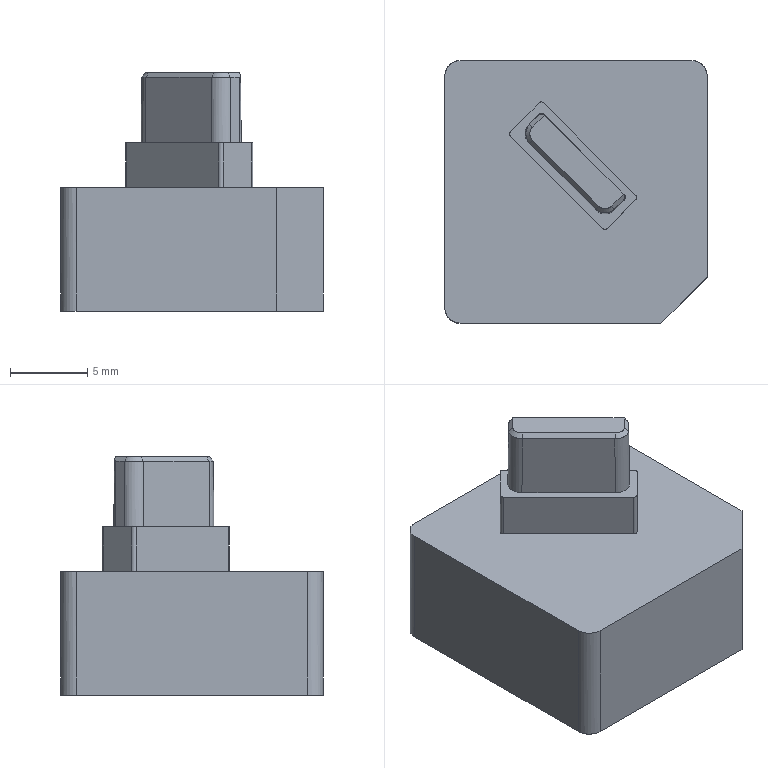NC program | PowerMill | posted with a generic post | part box 17 x 17 x 15.424 mm
Lines 1 to 1056 of 38437:
%
O0001
N104 ( POWERMILL CB  : 2026004.0)
N105 ( POST VER      : 2026.0.0.5161)
N106 ( OPTION FILE   : FANUC)
N107 ( OUTPUT WORKPLANE : WORLD)
N108 (  )
N109 ( TOOL LIST )
N110 (---------------------------------------)
N111 ( NO. | ID        | DIA.| TIP RAD|LENGTH)
N112 (---------------------------------------)
N113 (    1|D10C_1_1   |10.0 |  0.0   |70.88 )
N114 (    3|D10_1_1    |10.0 |  0.0   | 70.6 )
N115 (   14|D4_1_1     | 4.0 |  0.0   | 62.6 )
N116 (   13|TEXT_D4_1_1| 4.0 |  0.3   |62.68 )
N117 (---------------------------------------)
N118 (  )
N119 ( NUMBER OF TOOLPATHS: 10.0 )
N120 ( ESTIMATED PROGRAM DURATION: 0 HOURS 4 MIN 27 SEC)
N121 (  )
N122 G00 G21 G80 G40 G17
N123 G90
N124 G54
N125 G53 Z0.0
N126 (---------------)
N127 ( START TOOLPATH : 精公开粗01-扫面平行-D10C )
N128 (---------------)
N129 ( TOOL NO.    :1 )
N130 ( TOOL TYPE   : ENDMILL)
N131 ( TOOL ID     : D10C_1_1)
N132 ( TOOL DIA    : 10.0 LENGTH 70.88)
N133 T1
N134 M6
N135 S8000 M03
N136 G00 G90 X0.0 Y0.0
N137 G43 Z10.2 H1
N138
N139 G05 P10000 R4
N140 X11.28 Y11.28
N141 Z1.134
N142 G01 Z-0.066 F6000.0
N143 X-11.28 F10000.0
N144 Y5.64
N145 X11.28
N146 Y0.0
N147 X-11.28
N148 Y-5.64
N149 X11.28
N150 Y-11.28
N151 X-11.28
N152 X-16.28
N153 G00 Z10.2
N154 G05 P0
N155 (---------------)
N156 ( END TOOLPATH : 精公开粗01-扫面平行-D10C )
N157 (---------------)
N158 ( START TOOLPATH : 精公开粗01-外形偏置-D10C )
N159 (---------------)
N160 G00 X-0.181 Y1.1575 Z9.884
N161 G05 P10000 R4
N162 X16.993 Y4.7643
N163 Z0.7104
N164 G01 Z-0.4896 F6000.0
N165 X16.4655 F10000.0
N166 G03 X11.718 Y0.0168 I0.0 J-4.7475
N167 G01 Y-10.28
N168 G02 X10.718 Y-11.28 I-1.0 J0.0
N169 G01 X-11.08
N170 G02 X-12.08 Y-10.28 I0.0 J1.0
N171 G01 Y12.595
N172 G02 X-11.08 Y13.595 I1.0 J0.0
N173 G01 X10.718
N174 G02 X11.718 Y12.595 I0.0 J-1.0
N175 G01 Y0.0168
N176 X8.404 Y-0.196
N177 X8.4164 Y-0.3894
N178 X8.3267 Y-1.3785
N179 X8.1894 Y-1.9362
N180 X7.8985 Y-2.7096
N181 X7.5533 Y-3.3402
N182 X6.8288 Y-4.2565
N183 X6.0064 Y-5.075
N184 X5.233 Y-5.6668
N185 X5.0107 Y-5.8033
N186 X4.4596 Y-6.0808
N187 X3.6861 Y-6.3853
N188 X2.8628 Y-6.5768
N189 X2.1393 Y-6.649
N190 X1.3659 Y-6.6271
N191 X0.5924 Y-6.5194
N192 X-0.181 Y-6.3016
N193 X-0.9544 Y-5.9651
N194 X-1.2535 Y-5.8033
N195 X-1.7279 Y-5.4941
N196 X-2.2951 Y-5.0299
N197 X-2.5013 Y-4.8324
N198 X-6.171 Y-1.1628
N199 X-7.1418 Y-0.1514
N200 X-7.5329 Y0.3841
N201 X-7.9153 Y1.0674
N202 X-8.2576 Y1.9309
N203 X-8.4393 Y2.7044
N204 X-8.5261 Y3.4778
N205 X-8.5038 Y4.2512
N206 X-8.4011 Y5.0246
N207 X-8.1855 Y5.7981
N208 X-7.9153 Y6.4478
N209 X-7.3844 Y7.3449
N210 X-7.1418 Y7.664
N211 X-6.7331 Y8.1183
N212 X-5.9378 Y8.8918
N213 X-5.595 Y9.1738
N214 X-4.8222 Y9.6652
N215 X-4.0481 Y9.9937
N216 X-3.2747 Y10.1962
N217 X-2.5013 Y10.2908
N218 X-1.7279 Y10.2681
N219 X-0.9544 Y10.1475
N220 X-0.181 Y9.9029
N221 X0.3303 Y9.6652
N222 X0.5924 Y9.5152
N223 X1.3659 Y8.9732
N224 X2.1393 Y8.2277
N225 X6.8887 Y3.4778
N226 X7.4928 Y2.7044
N227 X7.9241 Y1.9309
N228 X8.2071 Y1.1575
N229 X8.3668 Y0.3841
N230 X8.404 Y-0.196
N231 X11.718 Y0.0168
N232 G00 Z3.3368
N233 G01 X16.993 Y4.7643
N234 G00 Z0.3368
N235 G01 Z-0.8632 F6000.0
N236 X16.4655 F10000.0
N237 G03 X11.718 Y0.0168 I0.0 J-4.7475
N238 G01 Y-10.28
N239 G02 X10.718 Y-11.28 I-1.0 J0.0
N240 G01 X-11.08
N241 G02 X-12.08 Y-10.28 I0.0 J1.0
N242 G01 Y12.595
N243 G02 X-11.08 Y13.595 I1.0 J0.0
N244 G01 X10.718
N245 G02 X11.718 Y12.595 I0.0 J-1.0
N246 G01 Y0.0239
N247 X8.4111 Y-0.196
N248 X8.424 Y-0.3894
N249 X8.3643 Y-1.1628
N250 X8.3328 Y-1.3101
N251 X8.3266 Y-1.3785
N252 X8.2632 Y-1.6361
N253 X8.1991 Y-1.9362
N254 X7.9038 Y-2.7096
N255 X7.5533 Y-3.3517
N256 X6.8433 Y-4.2565
N257 X6.0626 Y-5.0299
N258 X6.015 Y-5.0664
N259 X6.0064 Y-5.075
N260 X5.2793 Y-5.6313
N261 X5.233 Y-5.6668
N262 X5.231 Y-5.6679
N263 X5.0106 Y-5.8033
N264 X4.7463 Y-5.9364
N265 X4.4596 Y-6.0952
N266 X3.6861 Y-6.3853
N267 X2.8923 Y-6.5768
N268 X2.1393 Y-6.6513
N269 X1.3659 Y-6.6355
N270 X0.5924 Y-6.5238
N271 X-0.181 Y-6.3016
N272 X-0.9544 Y-5.9721
N273 X-1.2585 Y-5.8033
N274 X-1.7279 Y-5.4944
N275 X-2.3045 Y-5.0299
N276 X-2.5013 Y-4.8411
N277 X-6.3684 Y-0.9749
N278 X-6.9415 Y-0.3894
N279 X-7.1418 Y-0.1528
N280 X-7.5329 Y0.3841
N281 X-7.9153 Y1.052
N282 X-8.2576 Y1.9309
N283 X-8.4465 Y2.7044
N284 X-8.5286 Y3.4778
N285 X-8.5153 Y4.2512
N286 X-8.4055 Y5.0246
N287 X-8.1856 Y5.7981
N288 X-7.9153 Y6.4608
N289 X-7.3847 Y7.3449
N290 X-7.1418 Y7.6656
N291 X-6.7378 Y8.1183
N292 X-5.9501 Y8.8918
N293 X-5.595 Y9.1789
N294 X-4.8282 Y9.6652
N295 X-4.0481 Y10.0018
N296 X-3.2747 Y10.2057
N297 X-2.5013 Y10.2955
N298 X-1.7279 Y10.2743
N299 X-0.9544 Y10.1526
N300 X-0.181 Y9.9068
N301 X-0.0726 Y9.8524
N302 X0.3303 Y9.6651
N303 X0.5395 Y9.5454
N304 X0.5924 Y9.5189
N305 X1.3659 Y8.9797
N306 X2.1393 Y8.2347
N307 X6.8933 Y3.4778
N308 X7.499 Y2.7044
N309 X7.9275 Y1.9309
N310 X8.2137 Y1.1575
N311 X8.3726 Y0.3841
N312 X8.4111 Y-0.196
N313 X11.718 Y0.0239
N314 Y0.0168
N315 G00 Z2.9632
N316 G01 X16.993 Y4.7643
N317 G00 Z-0.0368
N318 G01 Z-1.2368 F6000.0
N319 X16.4655 F10000.0
N320 G03 X11.718 Y0.0168 I0.0 J-4.7475
N321 G01 Y-10.28
N322 G02 X10.718 Y-11.28 I-1.0 J0.0
N323 G01 X-11.08
N324 G02 X-12.08 Y-10.28 I0.0 J1.0
N325 G01 Y12.595
N326 G02 X-11.08 Y13.595 I1.0 J0.0
N327 G01 X10.718
N328 G02 X11.718 Y12.595 I0.0 J-1.0
N329 G01 Y0.0198
N330 X8.4151 Y-0.196
N331 X8.4277 Y-0.3894
N332 X8.3702 Y-1.1628
N333 X8.3286 Y-1.3561
N334 X8.3266 Y-1.3785
N335 X8.3044 Y-1.4688
N336 X8.2037 Y-1.9362
N337 X7.9091 Y-2.7096
N338 X7.5533 Y-3.3585
N339 X6.8479 Y-4.2565
N340 X6.0675 Y-5.0299
N341 X5.233 Y-5.6696
N342 X5.1815 Y-5.6983
N343 X5.0106 Y-5.8033
N344 X4.8222 Y-5.8981
N345 X4.4596 Y-6.0998
N346 X3.6861 Y-6.3854
N347 X2.9192 Y-6.5768
N348 X2.1393 Y-6.6536
N349 X1.3659 Y-6.6409
N350 X0.5924 Y-6.5284
N351 X-0.181 Y-6.3024
N352 X-0.9544 Y-5.978
N353 X-1.2661 Y-5.8033
N354 X-1.7279 Y-5.4946
N355 X-2.3103 Y-5.0299
N356 X-2.5013 Y-4.8467
N357 X-6.1852 Y-1.1628
N358 X-6.9467 Y-0.3894
N359 X-7.1418 Y-0.1583
N360 X-7.5353 Y0.3841
N361 X-7.9153 Y1.0427
N362 X-8.2577 Y1.9309
N363 X-8.4526 Y2.7044
N364 X-8.531 Y3.4778
N365 X-8.5199 Y4.2512
N366 X-8.4101 Y5.0246
N367 X-8.186 Y5.7981
N368 X-7.9153 Y6.4701
N369 X-7.385 Y7.3449
N370 X-7.1418 Y7.6711
N371 X-6.7424 Y8.1183
N372 X-5.9553 Y8.8918
N373 X-5.595 Y9.1838
N374 X-4.8345 Y9.6652
N375 X-4.0481 Y10.0064
N376 X-3.2747 Y10.2103
N377 X-2.5013 Y10.3002
N378 X-1.7279 Y10.2796
N379 X-0.9544 Y10.1573
N380 X-0.181 Y9.9114
N381 X0.0543 Y9.7934
N382 X0.3303 Y9.6651
N383 X0.4735 Y9.5831
N384 X0.5924 Y9.5235
N385 X1.3659 Y8.9843
N386 X2.1393 Y8.2393
N387 X6.8979 Y3.4778
N388 X7.5036 Y2.7044
N389 X7.9321 Y1.9309
N390 X8.2188 Y1.1575
N391 X8.3772 Y0.3841
N392 X8.4151 Y-0.196
N393 X11.718 Y0.0198
N394 Y0.0168
N395 G00 Z2.5896
N396 G01 X16.993 Y4.7643
N397 G00 Z-0.4104
N398 G01 Z-1.6104 F6000.0
N399 X16.4655 F10000.0
N400 G03 X11.718 Y0.0168 I0.0 J-4.7475
N401 G01 Y0.0156
N402 X8.419 Y-0.196
N403 X8.4314 Y-0.3894
N404 X8.3748 Y-1.1628
N405 X8.2083 Y-1.9362
N406 X7.9123 Y-2.7096
N407 X7.5533 Y-3.3651
N408 X6.8526 Y-4.2565
N409 X6.0725 Y-5.0299
N410 X5.233 Y-5.6742
N411 X5.1012 Y-5.7475
N412 X5.0106 Y-5.8032
N413 X4.9106 Y-5.8535
N414 X4.4596 Y-6.1044
N415 X3.6861 Y-6.3889
N416 X2.9447 Y-6.5768
N417 X2.1393 Y-6.6572
N418 X1.3659 Y-6.6455
N419 X0.5924 Y-6.533
N420 X-0.181 Y-6.307
N421 X-0.9544 Y-5.9826
N422 X-1.2737 Y-5.8033
N423 X-1.7279 Y-5.4967
N424 X-2.3152 Y-5.0299
N425 X-2.5013 Y-4.8513
N426 X-6.1898 Y-1.1628
N427 X-6.9512 Y-0.3894
N428 X-7.1418 Y-0.1637
N429 X-7.5399 Y0.3841
N430 X-7.9153 Y1.0334
N431 X-8.2609 Y1.9309
N432 X-8.4572 Y2.7044
N433 X-8.5346 Y3.4778
N434 X-8.5245 Y4.2512
N435 X-8.4147 Y5.0246
N436 X-8.1906 Y5.7981
N437 X-7.9153 Y6.4795
N438 X-7.3872 Y7.3449
N439 X-7.1418 Y7.6765
N440 X-6.747 Y8.1183
N441 X-5.9605 Y8.8918
N442 X-5.595 Y9.1884
N443 X-4.8408 Y9.6652
N444 X-4.0481 Y10.011
N445 X-3.2747 Y10.2149
N446 X-2.5013 Y10.3044
N447 X-1.7279 Y10.2842
N448 X-0.9544 Y10.162
N449 X-0.181 Y9.916
N450 X0.1813 Y9.7343
N451 X0.3302 Y9.6651
N452 X0.4076 Y9.6208
N453 X0.5924 Y9.5281
N454 X1.3659 Y8.9889
N455 X2.1393 Y8.2439
N456 X6.9025 Y3.4778
N457 X7.5082 Y2.7044
N458 X7.9367 Y1.9309
N459 X8.2234 Y1.1575
N460 X8.3818 Y0.3841
N461 X8.419 Y-0.196
N462 X11.718 Y0.0156
N463 Y-10.28
N464 G02 X10.718 Y-11.28 I-1.0 J0.0
N465 G01 X-11.08
N466 G02 X-12.08 Y-10.28 I0.0 J1.0
N467 G01 Y12.595
N468 G02 X-11.08 Y13.595 I1.0 J0.0
N469 G01 X10.718
N470 G02 X11.718 Y12.595 I0.0 J-1.0
N471 G01 Y0.0168
N472 G00 Z2.216
N473 G01 X16.993 Y4.7643
N474 G00 Z-0.784
N475 G01 Z-1.984 F6000.0
N476 X16.4655 F10000.0
N477 G03 X11.718 Y0.0168 I0.0 J-4.7475
N478 G01 Y0.0114
N479 X8.4229 Y-0.196
N480 X8.4351 Y-0.3894
N481 X8.3795 Y-1.1628
N482 X8.2129 Y-1.9362
N483 X7.9169 Y-2.7096
N484 X7.5533 Y-3.3718
N485 X6.8572 Y-4.2565
N486 X6.0774 Y-5.0299
N487 X5.233 Y-5.6789
N488 X5.0209 Y-5.7968
N489 X5.0106 Y-5.8032
N490 X4.9991 Y-5.8089
N491 X4.4596 Y-6.109
N492 X3.6861 Y-6.3935
N493 X2.9701 Y-6.5768
N494 X2.1393 Y-6.6618
N495 X1.3659 Y-6.6501
N496 X0.7874 Y-6.5768
N497 X0.6667 Y-6.5437
N498 X0.5924 Y-6.5329
N499 X0.073 Y-6.3812
N500 X-0.181 Y-6.3116
N501 X-0.9544 Y-5.9872
N502 X-1.2812 Y-5.8033
N503 X-1.7279 Y-5.5009
N504 X-2.3202 Y-5.0299
N505 X-2.5013 Y-4.8559
N506 X-6.1944 Y-1.1628
N507 X-6.9557 Y-0.3894
N508 X-6.9972 Y-0.3348
N509 X-7.1418 Y-0.1637
N510 X-7.4418 Y0.2491
N511 X-7.5445 Y0.3841
N512 X-7.9153 Y1.024
N513 X-8.2655 Y1.9309
N514 X-8.4618 Y2.7044
N515 X-8.5392 Y3.4778
N516 X-8.5291 Y4.2512
N517 X-8.4193 Y5.0246
N518 X-8.1952 Y5.7981
N519 X-7.9153 Y6.4888
N520 X-7.3914 Y7.3449
N521 X-7.1418 Y7.6819
N522 X-6.7516 Y8.1183
N523 X-5.9657 Y8.8918
N524 X-5.595 Y9.193
N525 X-4.8472 Y9.6652
N526 X-4.0481 Y10.0156
N527 X-3.2747 Y10.2196
N528 X-2.5013 Y10.3083
N529 X-1.7279 Y10.2888
N530 X-0.9544 Y10.1666
N531 X-0.181 Y9.9206
N532 X0.3083 Y9.6752
N533 X0.3302 Y9.665
N534 X0.3416 Y9.6585
N535 X0.5924 Y9.5327
N536 X1.3659 Y8.9935
N537 X2.1393 Y8.2485
N538 X6.9071 Y3.4778
N539 X7.5128 Y2.7044
N540 X7.9413 Y1.9309
N541 X8.228 Y1.1575
N542 X8.3864 Y0.3841
N543 X8.4229 Y-0.196
N544 X11.718 Y0.0114
N545 Y-10.28
N546 G02 X10.718 Y-11.28 I-1.0 J0.0
N547 G01 X-11.08
N548 G02 X-12.08 Y-10.28 I0.0 J1.0
N549 G01 Y12.595
N550 G02 X-11.08 Y13.595 I1.0 J0.0
N551 G01 X10.718
N552 G02 X11.718 Y12.595 I0.0 J-1.0
N553 G01 Y0.0168
N554 G00 Z1.8424
N555 G01 X16.993 Y4.7643
N556 G00 Z-1.1576
N557 G01 Z-2.3576 F6000.0
N558 X16.4655 F10000.0
N559 G03 X11.718 Y0.0168 I0.0 J-4.7475
N560 G01 Y0.0072
N561 X8.4268 Y-0.196
N562 X8.4387 Y-0.3894
N563 X8.3841 Y-1.1628
N564 X8.2175 Y-1.9362
N565 X7.9215 Y-2.7096
N566 X7.5533 Y-3.3784
N567 X6.8618 Y-4.2565
N568 X6.0823 Y-5.0299
N569 X5.233 Y-5.6835
N570 X4.4596 Y-6.1136
N571 X3.6861 Y-6.3982
N572 X2.9956 Y-6.5768
N573 X2.1393 Y-6.6664
N574 X1.3659 Y-6.6547
N575 X0.7622 Y-6.5768
N576 X0.6154 Y-6.5362
N577 X0.5924 Y-6.5329
N578 X0.404 Y-6.4778
N579 X-0.181 Y-6.3162
N580 X-0.9544 Y-5.9918
N581 X-1.2888 Y-5.8033
N582 X-1.7279 Y-5.5051
N583 X-2.3251 Y-5.0299
N584 X-2.5013 Y-4.8605
N585 X-6.199 Y-1.1628
N586 X-6.9602 Y-0.3894
N587 X-7.0434 Y-0.2801
N588 X-7.1418 Y-0.1637
N589 X-7.3446 Y0.1154
N590 X-7.5491 Y0.3841
N591 X-7.9153 Y1.0147
N592 X-8.2701 Y1.9309
N593 X-8.4664 Y2.7044
N594 X-8.5438 Y3.4778
N595 X-8.5337 Y4.2512
N596 X-8.4239 Y5.0246
N597 X-8.1998 Y5.7981
N598 X-7.9153 Y6.4981
N599 X-7.3956 Y7.3449
N600 X-7.1418 Y7.6874
N601 X-6.7562 Y8.1183
N602 X-5.9709 Y8.8918
N603 X-5.595 Y9.1976
N604 X-4.8535 Y9.6652
N605 X-4.0481 Y10.0202
N606 X-3.2747 Y10.2242
N607 X-2.5013 Y10.3123
N608 X-1.7279 Y10.2934
N609 X-0.9544 Y10.1712
N610 X-0.181 Y9.9252
N611 X0.5924 Y9.5373
N612 X1.3659 Y8.9982
N613 X2.1393 Y8.2532
N614 X6.9118 Y3.4778
N615 X7.5174 Y2.7044
N616 X7.946 Y1.9309
N617 X8.2326 Y1.1575
N618 X8.391 Y0.3841
N619 X8.4268 Y-0.196
N620 X11.718 Y0.0072
N621 Y-10.28
N622 G02 X10.718 Y-11.28 I-1.0 J0.0
N623 G01 X-11.08
N624 G02 X-12.08 Y-10.28 I0.0 J1.0
N625 G01 Y12.595
N626 G02 X-11.08 Y13.595 I1.0 J0.0
N627 G01 X10.718
N628 G02 X11.718 Y12.595 I0.0 J-1.0
N629 G01 Y0.0168
N630 G00 Z1.4688
N631 G01 X16.993 Y4.7643
N632 G00 Z-1.5312
N633 G01 Z-2.7312 F6000.0
N634 X16.4655 F10000.0
N635 G03 X11.718 Y0.0168 I0.0 J-4.7475
N636 G01 Y0.0029
N637 X8.4307 Y-0.196
N638 X8.4424 Y-0.3894
N639 X8.3887 Y-1.1628
N640 X8.2222 Y-1.9362
N641 X7.9261 Y-2.7096
N642 X7.5533 Y-3.3851
N643 X6.8664 Y-4.2565
N644 X6.0872 Y-5.0299
N645 X5.233 Y-5.6881
N646 X4.4596 Y-6.1182
N647 X3.6861 Y-6.4028
N648 X3.0199 Y-6.5768
N649 X2.1393 Y-6.671
N650 X1.3659 Y-6.6593
N651 X0.7371 Y-6.5768
N652 X-0.181 Y-6.3208
N653 X-0.9544 Y-5.9964
N654 X-1.2964 Y-5.8033
N655 X-1.7279 Y-5.5094
N656 X-2.33 Y-5.0299
N657 X-2.5013 Y-4.8651
N658 X-6.2036 Y-1.1628
N659 X-6.9647 Y-0.3894
N660 X-7.0897 Y-0.2252
N661 X-7.1417 Y-0.1636
N662 X-7.2482 Y-0.0171
N663 X-7.5538 Y0.3841
N664 X-7.9153 Y1.0053
N665 X-8.2747 Y1.9309
N666 X-8.4711 Y2.7044
N667 X-8.5484 Y3.4778
N668 X-8.5383 Y4.2512
N669 X-8.4285 Y5.0246
N670 X-8.2045 Y5.7981
N671 X-7.9153 Y6.5075
N672 X-7.4002 Y7.3449
N673 X-7.1418 Y7.6928
N674 X-6.7608 Y8.1183
N675 X-5.976 Y8.8918
N676 X-5.595 Y9.2022
N677 X-4.8598 Y9.6652
N678 X-4.0481 Y10.0248
N679 X-3.2747 Y10.2288
N680 X-2.5013 Y10.3163
N681 X-1.7279 Y10.298
N682 X-0.9544 Y10.1758
N683 X-0.181 Y9.9298
N684 X0.5924 Y9.5419
N685 X1.3659 Y9.0028
N686 X2.1393 Y8.2578
N687 X6.9164 Y3.4778
N688 X7.522 Y2.7044
N689 X7.9506 Y1.9309
N690 X8.2373 Y1.1575
N691 X8.3956 Y0.3841
N692 X8.4307 Y-0.196
N693 X11.718 Y0.0029
N694 Y-10.28
N695 G02 X10.718 Y-11.28 I-1.0 J0.0
N696 G01 X-11.08
N697 G02 X-12.08 Y-10.28 I0.0 J1.0
N698 G01 Y12.595
N699 G02 X-11.08 Y13.595 I1.0 J0.0
N700 G01 X10.718
N701 G02 X11.718 Y12.595 I0.0 J-1.0
N702 G01 Y0.0168
N703 G00 Z1.0952
N704 G01 X16.993 Y4.7643
N705 G00 Z-1.9048
N706 G01 Z-3.1048 F6000.0
N707 X16.4655 F10000.0
N708 G03 X11.718 Y0.0168 I0.0 J-4.7475
N709 G01 Y-0.0014
N710 X8.4346 Y-0.196
N711 X8.4461 Y-0.3894
N712 X8.3933 Y-1.1628
N713 X8.2268 Y-1.9362
N714 X7.9307 Y-2.7096
N715 X7.5533 Y-3.3918
N716 X6.871 Y-4.2565
N717 X6.0922 Y-5.0299
N718 X5.233 Y-5.6927
N719 X4.4596 Y-6.1228
N720 X3.6861 Y-6.4074
N721 X3.0429 Y-6.5768
N722 X2.1393 Y-6.6757
N723 X1.3659 Y-6.6639
N724 X0.7141 Y-6.5768
N725 X-0.181 Y-6.3254
N726 X-0.9544 Y-6.001
N727 X-1.3039 Y-5.8033
N728 X-1.7279 Y-5.514
N729 X-2.3349 Y-5.0299
N730 X-2.4672 Y-4.8978
N731 X-2.5012 Y-4.8651
N732 X-3.2744 Y-4.0919
N733 X-6.2082 Y-1.1628
N734 X-6.9692 Y-0.3894
N735 X-7.1362 Y-0.17
N736 X-7.1417 Y-0.1636
N737 X-7.1527 Y-0.1484
N738 X-7.5584 Y0.3841
N739 X-7.9153 Y0.996
N740 X-8.2793 Y1.9309
N741 X-8.4757 Y2.7044
N742 X-8.553 Y3.4778
N743 X-8.5429 Y4.2512
N744 X-8.4331 Y5.0246
N745 X-8.2091 Y5.7981
N746 X-7.9153 Y6.5168
N747 X-7.4048 Y7.3449
N748 X-7.1418 Y7.6982
N749 X-6.7654 Y8.1183
N750 X-5.9812 Y8.8918
N751 X-5.595 Y9.2068
N752 X-4.8669 Y9.6652
N753 X-4.0481 Y10.0295
N754 X-3.2747 Y10.2334
N755 X-2.5013 Y10.3203
N756 X-1.7279 Y10.3026
N757 X-0.9544 Y10.1804
N758 X-0.181 Y9.9344
N759 X0.5924 Y9.5465
N760 X1.3659 Y9.0074
N761 X2.1393 Y8.2624
N762 X6.921 Y3.4778
N763 X7.5267 Y2.7044
N764 X7.9552 Y1.9309
N765 X8.2419 Y1.1575
N766 X8.4002 Y0.3841
N767 X8.4346 Y-0.196
N768 X11.718 Y-0.0014
N769 Y-10.28
N770 G02 X10.718 Y-11.28 I-1.0 J0.0
N771 G01 X-11.08
N772 G02 X-12.08 Y-10.28 I0.0 J1.0
N773 G01 Y12.595
N774 G02 X-11.08 Y13.595 I1.0 J0.0
N775 G01 X10.718
N776 G02 X11.718 Y12.595 I0.0 J-1.0
N777 G01 Y0.0168
N778 G00 Z0.7216
N779 G01 X16.993 Y4.7643
N780 G00 Z-2.2784
N781 G01 Z-3.4784 F6000.0
N782 X16.4655 F10000.0
N783 G03 X11.718 Y0.0168 I0.0 J-4.7475
N784 G01 Y-0.0058
N785 X8.4385 Y-0.196
N786 X8.4497 Y-0.3894
N787 X8.3979 Y-1.1628
N788 X8.2314 Y-1.9362
N789 X7.9353 Y-2.7096
N790 X7.5533 Y-3.3984
N791 X6.8756 Y-4.2565
N792 X6.0971 Y-5.0299
N793 X5.233 Y-5.6973
N794 X4.4596 Y-6.1274
N795 X3.6861 Y-6.412
N796 X3.066 Y-6.5768
N797 X2.1393 Y-6.6803
N798 X1.3659 Y-6.6685
N799 X0.6916 Y-6.5768
N800 X-0.181 Y-6.33
N801 X-0.9544 Y-6.0056
N802 X-1.3114 Y-5.8033
N803 X-1.7279 Y-5.5186
N804 X-2.3398 Y-5.0299
N805 X-6.2129 Y-1.1628
N806 X-6.9737 Y-0.3894
N807 X-7.563 Y0.3841
N808 X-7.9153 Y0.9867
N809 X-8.2839 Y1.9309
N810 X-8.4803 Y2.7044
N811 X-8.5576 Y3.4778
N812 X-8.5476 Y4.2512
N813 X-8.4377 Y5.0246
N814 X-8.2137 Y5.7981
N815 X-7.9153 Y6.5261
N816 X-7.4094 Y7.3449
N817 X-7.1418 Y7.7036
N818 X-6.77 Y8.1183
N819 X-5.9863 Y8.8918
N820 X-5.595 Y9.2114
N821 X-4.8752 Y9.6652
N822 X-4.0481 Y10.0341
N823 X-3.2747 Y10.238
N824 X-2.5013 Y10.3242
N825 X-1.7279 Y10.3072
N826 X-0.9544 Y10.185
N827 X-0.181 Y9.9391
N828 X0.5924 Y9.5511
N829 X1.3659 Y9.012
N830 X2.1393 Y8.267
N831 X6.9256 Y3.4778
N832 X7.5313 Y2.7044
N833 X7.9598 Y1.9309
N834 X8.2465 Y1.1575
N835 X8.4048 Y0.3841
N836 X8.4385 Y-0.196
N837 X11.718 Y-0.0058
N838 Y-10.28
N839 G02 X10.718 Y-11.28 I-1.0 J0.0
N840 G01 X-11.08
N841 G02 X-12.08 Y-10.28 I0.0 J1.0
N842 G01 Y12.595
N843 G02 X-11.08 Y13.595 I1.0 J0.0
N844 G01 X10.718
N845 G02 X11.718 Y12.595 I0.0 J-1.0
N846 G01 Y0.0168
N847 G00 Z0.348
N848 G01 X16.993 Y4.7643
N849 G00 Z-2.652
N850 G01 Z-3.852 F6000.0
N851 X16.4655 F10000.0
N852 G03 X11.718 Y0.0168 I0.0 J-4.7475
N853 G01 Y-0.1071
N854 X8.4478 Y-0.2927
N855 X8.4533 Y-0.3894
N856 X8.4025 Y-1.1628
N857 X8.236 Y-1.9362
N858 X7.94 Y-2.7096
N859 X7.5533 Y-3.4051
N860 X6.8802 Y-4.2565
N861 X6.102 Y-5.0299
N862 X5.233 Y-5.7019
N863 X4.4596 Y-6.1321
N864 X3.6861 Y-6.4166
N865 X3.0891 Y-6.5768
N866 X2.1393 Y-6.6849
N867 X1.3659 Y-6.6732
N868 X0.6691 Y-6.5768
N869 X-0.181 Y-6.3347
N870 X-0.9544 Y-6.0102
N871 X-1.3188 Y-5.8033
N872 X-1.7279 Y-5.5232
N873 X-2.3447 Y-5.0299
N874 X-6.2175 Y-1.1628
N875 X-6.9781 Y-0.3894
N876 X-7.5676 Y0.3841
N877 X-7.9153 Y0.9773
N878 X-8.2885 Y1.9309
N879 X-8.4849 Y2.7044
N880 X-8.5622 Y3.4778
N881 X-8.5522 Y4.2512
N882 X-8.4424 Y5.0246
N883 X-8.2183 Y5.7981
N884 X-7.9153 Y6.5355
N885 X-7.414 Y7.3449
N886 X-7.1418 Y7.709
N887 X-6.7746 Y8.1183
N888 X-5.9914 Y8.8918
N889 X-5.595 Y9.2161
N890 X-4.8835 Y9.6652
N891 X-4.0481 Y10.0387
N892 X-3.2747 Y10.2426
N893 X-2.5013 Y10.3282
N894 X-1.7279 Y10.3118
N895 X-0.9544 Y10.1896
N896 X-0.181 Y9.9437
N897 X0.5924 Y9.5557
N898 X1.3659 Y9.0166
N899 X2.1393 Y8.2716
N900 X6.9302 Y3.4778
N901 X7.5359 Y2.7044
N902 X7.9644 Y1.9309
N903 X8.2511 Y1.1575
N904 X8.4094 Y0.3841
N905 X8.4478 Y-0.2927
N906 X11.718 Y-0.1071
N907 Y-10.28
N908 G02 X10.718 Y-11.28 I-1.0 J0.0
N909 G01 X-11.08
N910 G02 X-12.08 Y-10.28 I0.0 J1.0
N911 G01 Y12.595
N912 G02 X-11.08 Y13.595 I1.0 J0.0
N913 G01 X10.718
N914 G02 X11.718 Y12.595 I0.0 J-1.0
N915 G01 Y0.0168
N916 G00 Z-0.0256
N917 G01 X16.993 Y4.7643
N918 G00 Z-3.0256
N919 G01 Z-4.2256 F6000.0
N920 X16.4655 F10000.0
N921 G03 X11.718 Y0.0168 I0.0 J-4.7475
N922 G01 Y-0.1114
N923 X8.4516 Y-0.2927
N924 X8.457 Y-0.3894
N925 X8.4071 Y-1.1628
N926 X8.2406 Y-1.9362
N927 X7.9446 Y-2.7096
N928 X7.5533 Y-3.4117
N929 X6.8848 Y-4.2565
N930 X6.1069 Y-5.0299
N931 X5.233 Y-5.7065
N932 X4.4596 Y-6.1367
N933 X3.6861 Y-6.4212
N934 X3.1115 Y-6.5768
N935 X2.1393 Y-6.6895
N936 X1.3659 Y-6.6778
N937 X0.6466 Y-6.5768
N938 X-0.181 Y-6.3393
N939 X-0.9544 Y-6.0148
N940 X-1.3262 Y-5.8033
N941 X-1.7279 Y-5.5278
N942 X-2.3496 Y-5.0299
N943 X-6.2221 Y-1.1628
N944 X-6.9826 Y-0.3894
N945 X-7.5722 Y0.3841
N946 X-7.6779 Y0.5724
N947 X-7.9152 Y0.9773
N948 X-7.9383 Y1.0364
N949 X-8.0063 Y1.1575
N950 X-8.2932 Y1.9309
N951 X-8.4895 Y2.7044
N952 X-8.5668 Y3.4778
N953 X-8.5568 Y4.2512
N954 X-8.447 Y5.0246
N955 X-8.2229 Y5.7981
N956 X-7.9018 Y6.5715
N957 X-7.4186 Y7.3449
N958 X-7.1418 Y7.7144
N959 X-6.7793 Y8.1183
N960 X-5.9965 Y8.8918
N961 X-5.595 Y9.2207
N962 X-4.8918 Y9.6652
N963 X-4.0481 Y10.0433
N964 X-3.2747 Y10.2472
N965 X-2.5013 Y10.3321
N966 X-1.7279 Y10.3165
N967 X-0.9544 Y10.1942
N968 X-0.181 Y9.9483
N969 X0.5924 Y9.5604
N970 X1.3659 Y9.0212
N971 X2.1393 Y8.2762
N972 X6.9348 Y3.4778
N973 X7.5405 Y2.7044
N974 X7.969 Y1.9309
N975 X8.2557 Y1.1575
N976 X8.4141 Y0.3841
N977 X8.4516 Y-0.2927
N978 X11.718 Y-0.1114
N979 Y-10.28
N980 G02 X10.718 Y-11.28 I-1.0 J0.0
N981 G01 X-11.08
N982 G02 X-12.08 Y-10.28 I0.0 J1.0
N983 G01 Y12.595
N984 G02 X-11.08 Y13.595 I1.0 J0.0
N985 G01 X10.718
N986 G02 X11.718 Y12.595 I0.0 J-1.0
N987 G01 Y0.0168
N988 G00 Z-0.3992
N989 G01 X16.993 Y4.7643
N990 G00 Z-3.3992
N991 G01 Z-4.5992 F6000.0
N992 X16.4655 F10000.0
N993 G03 X11.718 Y0.0168 I0.0 J-4.7475
N994 G01 Y-0.113
N995 X8.4559 Y-0.2927
N996 X8.4613 Y-0.3894
N997 X8.4117 Y-1.1628
N998 X8.2452 Y-1.9362
N999 X7.9492 Y-2.7096
N1000 X7.5533 Y-3.4184
N1001 X6.8894 Y-4.2565
N1002 X6.1118 Y-5.0299
N1003 X5.233 Y-5.7111
N1004 X4.4596 Y-6.1413
N1005 X3.6861 Y-6.4258
N1006 X3.1332 Y-6.5768
N1007 X2.9127 Y-6.6194
N1008 X2.1393 Y-6.6941
N1009 X1.3659 Y-6.6824
N1010 X0.6241 Y-6.5768
N1011 X-0.181 Y-6.3439
N1012 X-0.9544 Y-6.0195
N1013 X-1.3336 Y-5.8033
N1014 X-1.7279 Y-5.5324
N1015 X-1.873 Y-5.4116
N1016 X-2.3496 Y-5.0299
N1017 X-2.4423 Y-4.9373
N1018 X-2.5013 Y-4.8882
N1019 X-6.2267 Y-1.1628
N1020 X-6.9871 Y-0.3894
N1021 X-7.5768 Y0.3841
N1022 X-7.7883 Y0.7608
N1023 X-7.9152 Y0.9774
N1024 X-7.9275 Y1.009
N1025 X-8.0109 Y1.1575
N1026 X-8.2978 Y1.9309
N1027 X-8.4941 Y2.7044
N1028 X-8.5714 Y3.4778
N1029 X-8.5614 Y4.2512
N1030 X-8.4516 Y5.0246
N1031 X-8.2275 Y5.7981
N1032 X-7.9153 Y6.5541
N1033 X-7.4232 Y7.3449
N1034 X-7.1418 Y7.7198
N1035 X-6.7839 Y8.1183
N1036 X-6.0016 Y8.8918
N1037 X-5.595 Y9.2253
N1038 X-4.9001 Y9.6652
N1039 X-4.0481 Y10.0479
N1040 X-3.2747 Y10.2518
N1041 X-2.5013 Y10.3361
N1042 X-1.7279 Y10.3211
N1043 X-0.9544 Y10.1988
N1044 X-0.181 Y9.9529
N1045 X0.4179 Y9.6652
N1046 X0.5184 Y9.5974
N1047 X0.5924 Y9.5603
N1048 X1.1589 Y9.1654
N1049 X1.3659 Y9.0258
N1050 X2.1393 Y8.2808
N1051 X6.9394 Y3.4778
N1052 X7.5451 Y2.7044
N1053 X7.9736 Y1.9309
N1054 X8.2603 Y1.1575
N1055 X8.4187 Y0.3841
N1056 X8.4559 Y-0.2927
N1057 X11.718 Y-0.113
N1058 Y-10.28
N1059 G02 X10.718 Y-11.28 I-1.0 J0.0
N1060 G01 X-11.08
N1061 G02 X-12.08 Y-10.28 I0.0 J1.0
N1062 G01 Y12.595
N1063 G02 X-11.08 Y13.595 I1.0 J0.0
N1064 G01 X10.718
N1065 G02 X11.718 Y12.595 I0.0 J-1.0
N1066 G01 Y0.0168
N1067 G00 Z-0.753
N1068 G01 X16.993 Y4.7643
N1069 G00 Z-3.753
N1070 G01 Z-4.953 F6000.0
N1071 X16.4655 F10000.0
N1072 G03 X11.718 Y0.0168 I0.0 J-4.7475
N1073 G01 Y-10.28
N1074 G02 X10.718 Y-11.28 I-1.0 J0.0
N1075 G01 X-11.08
N1076 G02 X-12.08 Y-10.28 I0.0 J1.0
N1077 G01 Y3.5224
N1078 X-9.5727 Y3.4778
N1079 X-9.559 Y4.2512
N1080 X-9.4621 Y4.9064
N1081 X-9.1885 Y5.7981
N1082 X-8.7988 Y6.5715
N1083 X-8.2453 Y7.3449
N1084 X-5.9373 Y9.6652
N1085 X-5.595 Y9.9513
N1086 X-4.8399 Y10.4386
N1087 X-4.0481 Y10.7928
N1088 X-3.2747 Y11.0008
N1089 X-2.5013 Y11.0888
N1090 X-1.7279 Y11.0727
N1091 X-0.9544 Y10.9464
N1092 X-0.181 Y10.6964
N1093 X0.5924 Y10.3033
N1094 X1.3659 Y9.7447
N1095 X2.1393 Y8.9892
N1096 X7.6505 Y3.4778
N1097 X8.2783 Y2.7044
N1098 X8.7158 Y1.9309
N1099 X9.0067 Y1.1575
N1100 X9.1691 Y0.3841
N1101 X9.2151 Y-0.3894
N1102 X9.1619 Y-1.1628
N1103 X8.9913 Y-1.9362
N1104 X8.6909 Y-2.7096
N1105 X8.3267 Y-3.3569
N1106 X7.5986 Y-4.2565
N1107 X6.0064 Y-5.8487
N1108 X5.233 Y-6.5579
N1109 X4.4596 Y-7.0553
N1110 X3.8205 Y-7.3502
N1111 X2.9127 Y-7.6076
N1112 X2.1393 Y-7.6957
N1113 X1.3659 Y-7.6797
N1114 X0.5924 Y-7.5535
N1115 X-0.0632 Y-7.3502
N1116 X-0.9544 Y-6.9104
N1117 X-1.4511 Y-6.5768
N1118 X-1.7279 Y-6.3519
N1119 X-2.2946 Y-5.8033
N1120 X-7.9153 Y-0.1826
N1121 X-8.4219 Y0.3841
N1122 X-8.6887 Y0.762
N1123 X-8.9232 Y1.1575
N1124 X-9.2709 Y1.9309
N1125 X-9.4621 Y2.6063
N1126 X-9.5727 Y3.4778
N1127 X-12.08 Y3.5224
N1128 Y12.595
N1129 G02 X-11.08 Y13.595 I1.0 J0.0
N1130 G01 X10.718
N1131 G02 X11.718 Y12.595 I0.0 J-1.0
N1132 G01 Y0.0168
N1133 G00 Z-1.1069
N1134 G01 X16.993 Y4.7643
N1135 G00 Z-4.1069
N1136 G01 Z-5.3069 F6000.0
N1137 X16.4655 F10000.0
N1138 G03 X11.718 Y0.0168 I0.0 J-4.7475
N1139 G01 Y-10.28
N1140 G02 X10.718 Y-11.28 I-1.0 J0.0
N1141 G01 X-11.08
N1142 G02 X-12.08 Y-10.28 I0.0 J1.0
N1143 G01 Y3.5224
N1144 X-9.5727 Y3.4778
N1145 X-9.559 Y4.2512
N1146 X-9.4621 Y4.9064
N1147 X-9.1886 Y5.7981
N1148 X-8.7988 Y6.5715
N1149 X-8.2453 Y7.3449
N1150 X-5.9373 Y9.6652
N1151 X-5.595 Y9.9514
N1152 X-4.8399 Y10.4386
N1153 X-4.0481 Y10.7928